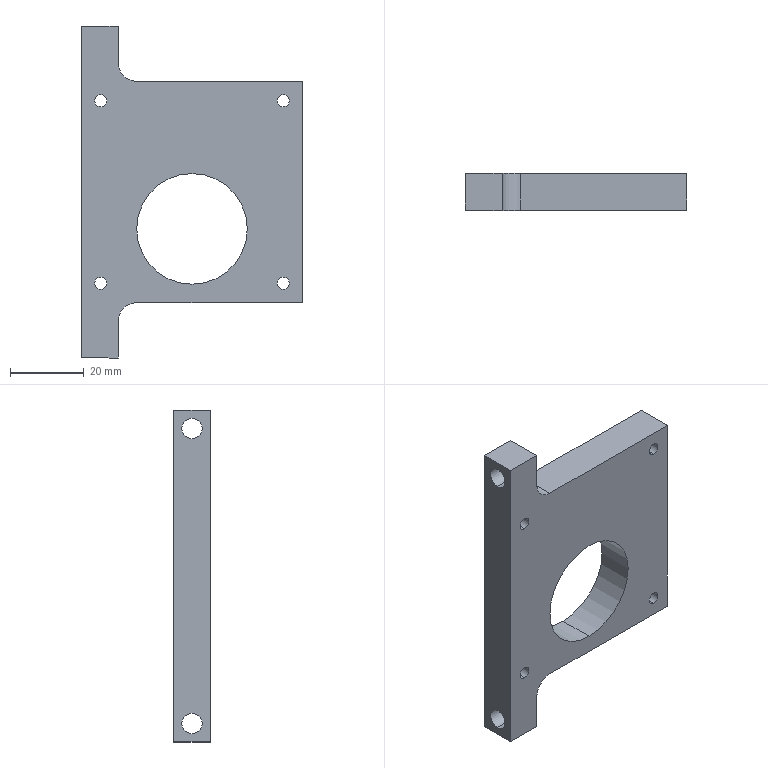Part | SolidWorks | features HoleWzd 3, Cut 1, Extrusion 1, Fillet 1, ICE 1, MoveFace 1 | 1 solid | 30 faces | box 60 x 10 x 90 mm | volume 31044 mm3 | cylinder 18 | plane 10 | cone 2 | commonest cylinder face diameters 3.3 x8 5.5 x4 4.2 x2 10 x2 30 x2
STEP:
#1=CARTESIAN_POINT('',(17.6,4.5,12.101));
#2=VERTEX_POINT('',#1);
#3=CARTESIAN_POINT('',(17.6,4.5,7.901));
#4=VERTEX_POINT('',#3);
#5=CARTESIAN_POINT('',(17.6,4.5,10.001));
#6=DIRECTION('',(1.,0.,0.));
#7=DIRECTION('',(0.,0.,-1.));
#8=AXIS2_PLACEMENT_3D('',#5,#6,#7);
#9=CIRCLE('',#8,2.1);
#10=EDGE_CURVE('',#2,#4,#9,.T.);
#11=ORIENTED_EDGE('',*,*,#10,.F.);
#12=CARTESIAN_POINT('',(30.,4.5,12.101));
#13=VERTEX_POINT('',#12);
#14=CARTESIAN_POINT('',(30.,4.5,12.101));
#15=DIRECTION('',(1.,0.,0.));
#16=VECTOR('',#15,1000.);
#17=LINE('',#14,#16);
#18=EDGE_CURVE('',#2,#13,#17,.T.);
#19=ORIENTED_EDGE('',*,*,#18,.T.);
#20=CARTESIAN_POINT('',(30.,4.5,7.901));
#21=VERTEX_POINT('',#20);
#22=CARTESIAN_POINT('',(30.,4.5,10.001));
#23=DIRECTION('',(1.,0.,0.));
#24=DIRECTION('',(0.,0.,-1.));
#25=AXIS2_PLACEMENT_3D('',#22,#23,#24);
#26=CIRCLE('',#25,2.1);
#27=EDGE_CURVE('',#13,#21,#26,.T.);
#28=ORIENTED_EDGE('',*,*,#27,.T.);
#29=CARTESIAN_POINT('',(30.,4.5,7.901));
#30=DIRECTION('',(1.,0.,0.));
#31=VECTOR('',#30,1000.);
#32=LINE('',#29,#31);
#33=EDGE_CURVE('',#4,#21,#32,.T.);
#34=ORIENTED_EDGE('',*,*,#33,.F.);
#35=EDGE_LOOP('',(#11,#19,#28,#34));
#36=FACE_OUTER_BOUND('',#35,.T.);
#37=CARTESIAN_POINT('',(30.,4.5,10.001));
#38=DIRECTION('',(1.,0.,0.));
#39=DIRECTION('',(0.,0.,-1.));
#40=AXIS2_PLACEMENT_3D('',#37,#38,#39);
#41=CYLINDRICAL_SURFACE('',#40,2.1);
#42=ADVANCED_FACE('',(#36),#41,.F.);
#43=CARTESIAN_POINT('',(16.338,4.5,10.001));
#44=VERTEX_POINT('',#43);
#45=CARTESIAN_POINT('',(17.6,4.5,7.901));
#46=DIRECTION('',(0.515,0.,-0.8572));
#47=VECTOR('',#46,1000.);
#48=LINE('',#45,#47);
#49=EDGE_CURVE('',#44,#4,#48,.T.);
#50=ORIENTED_EDGE('',*,*,#49,.F.);
#51=CARTESIAN_POINT('',(17.6,4.5,12.101));
#52=DIRECTION('',(0.515,0.,0.8572));
#53=VECTOR('',#52,1000.);
#54=LINE('',#51,#53);
#55=EDGE_CURVE('',#44,#2,#54,.T.);
#56=ORIENTED_EDGE('',*,*,#55,.T.);
#57=ORIENTED_EDGE('',*,*,#10,.T.);
#58=EDGE_LOOP('',(#50,#56,#57));
#59=FACE_OUTER_BOUND('',#58,.T.);
#60=CARTESIAN_POINT('',(17.6,4.5,10.001));
#61=DIRECTION('',(1.,0.,0.));
#62=DIRECTION('',(0.,0.,-1.));
#63=AXIS2_PLACEMENT_3D('',#60,#61,#62);
#64=CONICAL_SURFACE('',#63,2.1,1.03);
#65=ADVANCED_FACE('',(#59),#64,.F.);
#66=CARTESIAN_POINT('',(-20.,5.,-42.75));
#67=VERTEX_POINT('',#66);
#68=CARTESIAN_POINT('',(-20.,5.,-37.25));
#69=VERTEX_POINT('',#68);
#70=CARTESIAN_POINT('',(-20.,5.,-40.));
#71=DIRECTION('',(-1.,0.,0.));
#72=DIRECTION('',(0.,0.,1.));
#73=AXIS2_PLACEMENT_3D('',#70,#71,#72);
#74=CIRCLE('',#73,2.75);
#75=EDGE_CURVE('',#67,#69,#74,.T.);
#76=ORIENTED_EDGE('',*,*,#75,.F.);
#77=CARTESIAN_POINT('',(-30.,5.,-42.75));
#78=VERTEX_POINT('',#77);
#79=CARTESIAN_POINT('',(-30.,5.,-42.75));
#80=DIRECTION('',(-1.,0.,0.));
#81=VECTOR('',#80,1000.);
#82=LINE('',#79,#81);
#83=EDGE_CURVE('',#67,#78,#82,.T.);
#84=ORIENTED_EDGE('',*,*,#83,.T.);
#85=CARTESIAN_POINT('',(-30.,5.,-37.25));
#86=VERTEX_POINT('',#85);
#87=CARTESIAN_POINT('',(-30.,5.,-40.));
#88=DIRECTION('',(-1.,0.,0.));
#89=DIRECTION('',(0.,0.,1.));
#90=AXIS2_PLACEMENT_3D('',#87,#88,#89);
#91=CIRCLE('',#90,2.75);
#92=EDGE_CURVE('',#78,#86,#91,.T.);
#93=ORIENTED_EDGE('',*,*,#92,.T.);
#94=CARTESIAN_POINT('',(-30.,5.,-37.25));
#95=DIRECTION('',(-1.,0.,0.));
#96=VECTOR('',#95,1000.);
#97=LINE('',#94,#96);
#98=EDGE_CURVE('',#69,#86,#97,.T.);
#99=ORIENTED_EDGE('',*,*,#98,.F.);
#100=EDGE_LOOP('',(#76,#84,#93,#99));
#101=FACE_OUTER_BOUND('',#100,.T.);
#102=CARTESIAN_POINT('',(-30.,5.,-40.));
#103=DIRECTION('',(-1.,0.,0.));
#104=DIRECTION('',(0.,0.,1.));
#105=AXIS2_PLACEMENT_3D('',#102,#103,#104);
#106=CYLINDRICAL_SURFACE('',#105,2.75);
#107=ADVANCED_FACE('',(#101),#106,.F.);
#108=CARTESIAN_POINT('',(-20.,5.,37.25));
#109=VERTEX_POINT('',#108);
#110=CARTESIAN_POINT('',(-20.,5.,42.75));
#111=VERTEX_POINT('',#110);
#112=CARTESIAN_POINT('',(-20.,5.,40.));
#113=DIRECTION('',(-1.,0.,0.));
#114=DIRECTION('',(0.,0.,1.));
#115=AXIS2_PLACEMENT_3D('',#112,#113,#114);
#116=CIRCLE('',#115,2.75);
#117=EDGE_CURVE('',#109,#111,#116,.T.);
#118=ORIENTED_EDGE('',*,*,#117,.F.);
#119=CARTESIAN_POINT('',(-30.,5.,37.25));
#120=VERTEX_POINT('',#119);
#121=CARTESIAN_POINT('',(-30.,5.,37.25));
#122=DIRECTION('',(-1.,0.,0.));
#123=VECTOR('',#122,1000.);
#124=LINE('',#121,#123);
#125=EDGE_CURVE('',#109,#120,#124,.T.);
#126=ORIENTED_EDGE('',*,*,#125,.T.);
#127=CARTESIAN_POINT('',(-30.,5.,42.75));
#128=VERTEX_POINT('',#127);
#129=CARTESIAN_POINT('',(-30.,5.,40.));
#130=DIRECTION('',(-1.,0.,0.));
#131=DIRECTION('',(0.,0.,1.));
#132=AXIS2_PLACEMENT_3D('',#129,#130,#131);
#133=CIRCLE('',#132,2.75);
#134=EDGE_CURVE('',#120,#128,#133,.T.);
#135=ORIENTED_EDGE('',*,*,#134,.T.);
#136=CARTESIAN_POINT('',(-30.,5.,42.75));
#137=DIRECTION('',(-1.,0.,0.));
#138=VECTOR('',#137,1000.);
#139=LINE('',#136,#138);
#140=EDGE_CURVE('',#111,#128,#139,.T.);
#141=ORIENTED_EDGE('',*,*,#140,.F.);
#142=EDGE_LOOP('',(#118,#126,#135,#141));
#143=FACE_OUTER_BOUND('',#142,.T.);
#144=CARTESIAN_POINT('',(-30.,5.,40.));
#145=DIRECTION('',(-1.,0.,0.));
#146=DIRECTION('',(0.,0.,1.));
#147=AXIS2_PLACEMENT_3D('',#144,#145,#146);
#148=CYLINDRICAL_SURFACE('',#147,2.75);
#149=ADVANCED_FACE('',(#143),#148,.F.);
#150=CARTESIAN_POINT('',(-24.749,10.,26.397));
#151=VERTEX_POINT('',#150);
#152=CARTESIAN_POINT('',(-24.749,10.,23.097));
#153=VERTEX_POINT('',#152);
#154=CARTESIAN_POINT('',(-24.749,10.,24.747));
#155=DIRECTION('',(0.,-1.,0.));
#156=DIRECTION('',(0.,0.,-1.));
#157=AXIS2_PLACEMENT_3D('',#154,#155,#156);
#158=CIRCLE('',#157,1.65);
#159=EDGE_CURVE('',#151,#153,#158,.T.);
#160=ORIENTED_EDGE('',*,*,#159,.F.);
#161=CARTESIAN_POINT('',(-24.749,0.,26.397));
#162=VERTEX_POINT('',#161);
#163=CARTESIAN_POINT('',(-24.749,0.,26.397));
#164=DIRECTION('',(0.,-1.,0.));
#165=VECTOR('',#164,1000.);
#166=LINE('',#163,#165);
#167=EDGE_CURVE('',#151,#162,#166,.T.);
#168=ORIENTED_EDGE('',*,*,#167,.T.);
#169=CARTESIAN_POINT('',(-24.749,0.,23.097));
#170=VERTEX_POINT('',#169);
#171=CARTESIAN_POINT('',(-24.749,0.,24.747));
#172=DIRECTION('',(0.,-1.,0.));
#173=DIRECTION('',(0.,0.,-1.));
#174=AXIS2_PLACEMENT_3D('',#171,#172,#173);
#175=CIRCLE('',#174,1.65);
#176=EDGE_CURVE('',#162,#170,#175,.T.);
#177=ORIENTED_EDGE('',*,*,#176,.T.);
#178=CARTESIAN_POINT('',(-24.749,0.,23.097));
#179=DIRECTION('',(0.,-1.,0.));
#180=VECTOR('',#179,1000.);
#181=LINE('',#178,#180);
#182=EDGE_CURVE('',#153,#170,#181,.T.);
#183=ORIENTED_EDGE('',*,*,#182,.F.);
#184=EDGE_LOOP('',(#160,#168,#177,#183));
#185=FACE_OUTER_BOUND('',#184,.T.);
#186=CARTESIAN_POINT('',(-24.749,0.,24.747));
#187=DIRECTION('',(0.,-1.,0.));
#188=DIRECTION('',(0.,0.,-1.));
#189=AXIS2_PLACEMENT_3D('',#186,#187,#188);
#190=CYLINDRICAL_SURFACE('',#189,1.65);
#191=ADVANCED_FACE('',(#185),#190,.F.);
#192=CARTESIAN_POINT('',(-24.749,10.,-23.1));
#193=VERTEX_POINT('',#192);
#194=CARTESIAN_POINT('',(-24.749,10.,-26.4));
#195=VERTEX_POINT('',#194);
#196=CARTESIAN_POINT('',(-24.749,10.,-24.75));
#197=DIRECTION('',(0.,-1.,0.));
#198=DIRECTION('',(0.,0.,-1.));
#199=AXIS2_PLACEMENT_3D('',#196,#197,#198);
#200=CIRCLE('',#199,1.65);
#201=EDGE_CURVE('',#193,#195,#200,.T.);
#202=ORIENTED_EDGE('',*,*,#201,.F.);
#203=CARTESIAN_POINT('',(-24.749,0.,-23.1));
#204=VERTEX_POINT('',#203);
#205=CARTESIAN_POINT('',(-24.749,0.,-23.1));
#206=DIRECTION('',(0.,-1.,0.));
#207=VECTOR('',#206,1000.);
#208=LINE('',#205,#207);
#209=EDGE_CURVE('',#193,#204,#208,.T.);
#210=ORIENTED_EDGE('',*,*,#209,.T.);
#211=CARTESIAN_POINT('',(-24.749,0.,-26.4));
#212=VERTEX_POINT('',#211);
#213=CARTESIAN_POINT('',(-24.749,0.,-24.75));
#214=DIRECTION('',(0.,-1.,0.));
#215=DIRECTION('',(0.,0.,-1.));
#216=AXIS2_PLACEMENT_3D('',#213,#214,#215);
#217=CIRCLE('',#216,1.65);
#218=EDGE_CURVE('',#204,#212,#217,.T.);
#219=ORIENTED_EDGE('',*,*,#218,.T.);
#220=CARTESIAN_POINT('',(-24.749,0.,-26.4));
#221=DIRECTION('',(0.,-1.,0.));
#222=VECTOR('',#221,1000.);
#223=LINE('',#220,#222);
#224=EDGE_CURVE('',#195,#212,#223,.T.);
#225=ORIENTED_EDGE('',*,*,#224,.F.);
#226=EDGE_LOOP('',(#202,#210,#219,#225));
#227=FACE_OUTER_BOUND('',#226,.T.);
#228=CARTESIAN_POINT('',(-24.749,0.,-24.75));
#229=DIRECTION('',(0.,-1.,0.));
#230=DIRECTION('',(0.,0.,-1.));
#231=AXIS2_PLACEMENT_3D('',#228,#229,#230);
#232=CYLINDRICAL_SURFACE('',#231,1.65);
#233=ADVANCED_FACE('',(#227),#232,.F.);
#234=CARTESIAN_POINT('',(24.749,10.,-23.1));
#235=VERTEX_POINT('',#234);
#236=CARTESIAN_POINT('',(24.749,10.,-26.4));
#237=VERTEX_POINT('',#236);
#238=CARTESIAN_POINT('',(24.749,10.,-24.75));
#239=DIRECTION('',(0.,-1.,0.));
#240=DIRECTION('',(0.,0.,-1.));
#241=AXIS2_PLACEMENT_3D('',#238,#239,#240);
#242=CIRCLE('',#241,1.65);
#243=EDGE_CURVE('',#235,#237,#242,.T.);
#244=ORIENTED_EDGE('',*,*,#243,.F.);
#245=CARTESIAN_POINT('',(24.749,0.,-23.1));
#246=VERTEX_POINT('',#245);
#247=CARTESIAN_POINT('',(24.749,0.,-23.1));
#248=DIRECTION('',(0.,-1.,0.));
#249=VECTOR('',#248,1000.);
#250=LINE('',#247,#249);
#251=EDGE_CURVE('',#235,#246,#250,.T.);
#252=ORIENTED_EDGE('',*,*,#251,.T.);
#253=CARTESIAN_POINT('',(24.749,0.,-26.4));
#254=VERTEX_POINT('',#253);
#255=CARTESIAN_POINT('',(24.749,0.,-24.75));
#256=DIRECTION('',(0.,-1.,0.));
#257=DIRECTION('',(0.,0.,-1.));
#258=AXIS2_PLACEMENT_3D('',#255,#256,#257);
#259=CIRCLE('',#258,1.65);
#260=EDGE_CURVE('',#246,#254,#259,.T.);
#261=ORIENTED_EDGE('',*,*,#260,.T.);
#262=CARTESIAN_POINT('',(24.749,0.,-26.4));
#263=DIRECTION('',(0.,-1.,0.));
#264=VECTOR('',#263,1000.);
#265=LINE('',#262,#264);
#266=EDGE_CURVE('',#237,#254,#265,.T.);
#267=ORIENTED_EDGE('',*,*,#266,.F.);
#268=EDGE_LOOP('',(#244,#252,#261,#267));
#269=FACE_OUTER_BOUND('',#268,.T.);
#270=CARTESIAN_POINT('',(24.749,0.,-24.75));
#271=DIRECTION('',(0.,-1.,0.));
#272=DIRECTION('',(0.,0.,-1.));
#273=AXIS2_PLACEMENT_3D('',#270,#271,#272);
#274=CYLINDRICAL_SURFACE('',#273,1.65);
#275=ADVANCED_FACE('',(#269),#274,.F.);
#276=CARTESIAN_POINT('',(24.749,10.,26.397));
#277=VERTEX_POINT('',#276);
#278=CARTESIAN_POINT('',(24.749,10.,23.097));
#279=VERTEX_POINT('',#278);
#280=CARTESIAN_POINT('',(24.749,10.,24.747));
#281=DIRECTION('',(0.,-1.,0.));
#282=DIRECTION('',(0.,0.,-1.));
#283=AXIS2_PLACEMENT_3D('',#280,#281,#282);
#284=CIRCLE('',#283,1.65);
#285=EDGE_CURVE('',#277,#279,#284,.T.);
#286=ORIENTED_EDGE('',*,*,#285,.F.);
#287=CARTESIAN_POINT('',(24.749,0.,26.397));
#288=VERTEX_POINT('',#287);
#289=CARTESIAN_POINT('',(24.749,0.,26.397));
#290=DIRECTION('',(0.,-1.,0.));
#291=VECTOR('',#290,1000.);
#292=LINE('',#289,#291);
#293=EDGE_CURVE('',#277,#288,#292,.T.);
#294=ORIENTED_EDGE('',*,*,#293,.T.);
#295=CARTESIAN_POINT('',(24.749,0.,23.097));
#296=VERTEX_POINT('',#295);
#297=CARTESIAN_POINT('',(24.749,0.,24.747));
#298=DIRECTION('',(0.,-1.,0.));
#299=DIRECTION('',(0.,0.,-1.));
#300=AXIS2_PLACEMENT_3D('',#297,#298,#299);
#301=CIRCLE('',#300,1.65);
#302=EDGE_CURVE('',#288,#296,#301,.T.);
#303=ORIENTED_EDGE('',*,*,#302,.T.);
#304=CARTESIAN_POINT('',(24.749,0.,23.097));
#305=DIRECTION('',(0.,-1.,0.));
#306=VECTOR('',#305,1000.);
#307=LINE('',#304,#306);
#308=EDGE_CURVE('',#279,#296,#307,.T.);
#309=ORIENTED_EDGE('',*,*,#308,.F.);
#310=EDGE_LOOP('',(#286,#294,#303,#309));
#311=FACE_OUTER_BOUND('',#310,.T.);
#312=CARTESIAN_POINT('',(24.749,0.,24.747));
#313=DIRECTION('',(0.,-1.,0.));
#314=DIRECTION('',(0.,0.,-1.));
#315=AXIS2_PLACEMENT_3D('',#312,#313,#314);
#316=CYLINDRICAL_SURFACE('',#315,1.65);
#317=ADVANCED_FACE('',(#311),#316,.F.);
#318=CARTESIAN_POINT('',(0.,10.,5.));
#319=VERTEX_POINT('',#318);
#320=CARTESIAN_POINT('',(0.,10.,-25.));
#321=VERTEX_POINT('',#320);
#322=CARTESIAN_POINT('',(0.,10.,-10.));
#323=DIRECTION('',(0.,-1.,0.));
#324=DIRECTION('',(0.,0.,-1.));
#325=AXIS2_PLACEMENT_3D('',#322,#323,#324);
#326=CIRCLE('',#325,15.);
#327=EDGE_CURVE('',#319,#321,#326,.T.);
#328=ORIENTED_EDGE('',*,*,#327,.F.);
#329=CARTESIAN_POINT('',(0.,0.,5.));
#330=VERTEX_POINT('',#329);
#331=CARTESIAN_POINT('',(0.,10.,5.));
#332=DIRECTION('',(0.,-1.,0.));
#333=VECTOR('',#332,1000.);
#334=LINE('',#331,#333);
#335=EDGE_CURVE('',#319,#330,#334,.T.);
#336=ORIENTED_EDGE('',*,*,#335,.T.);
#337=CARTESIAN_POINT('',(0.,0.,-25.));
#338=VERTEX_POINT('',#337);
#339=CARTESIAN_POINT('',(0.,0.,-10.));
#340=DIRECTION('',(0.,-1.,0.));
#341=DIRECTION('',(0.,0.,-1.));
#342=AXIS2_PLACEMENT_3D('',#339,#340,#341);
#343=CIRCLE('',#342,15.);
#344=EDGE_CURVE('',#330,#338,#343,.T.);
#345=ORIENTED_EDGE('',*,*,#344,.T.);
#346=CARTESIAN_POINT('',(0.,10.,-25.));
#347=DIRECTION('',(0.,-1.,0.));
#348=VECTOR('',#347,1000.);
#349=LINE('',#346,#348);
#350=EDGE_CURVE('',#321,#338,#349,.T.);
#351=ORIENTED_EDGE('',*,*,#350,.F.);
#352=EDGE_LOOP('',(#328,#336,#345,#351));
#353=FACE_OUTER_BOUND('',#352,.T.);
#354=CARTESIAN_POINT('',(0.,10.,-10.));
#355=DIRECTION('',(0.,-1.,0.));
#356=DIRECTION('',(0.,0.,-1.));
#357=AXIS2_PLACEMENT_3D('',#354,#355,#356);
#358=CYLINDRICAL_SURFACE('',#357,15.);
#359=ADVANCED_FACE('',(#353),#358,.F.);
#360=CARTESIAN_POINT('',(-30.,5.,-40.));
#361=DIRECTION('',(-1.,0.,0.));
#362=DIRECTION('',(0.,0.,1.));
#363=AXIS2_PLACEMENT_3D('',#360,#361,#362);
#364=CIRCLE('',#363,2.75);
#365=EDGE_CURVE('',#86,#78,#364,.T.);
#366=ORIENTED_EDGE('',*,*,#365,.F.);
#367=ORIENTED_EDGE('',*,*,#92,.F.);
#368=EDGE_LOOP('',(#366,#367));
#369=FACE_BOUND('',#368,.T.);
#370=CARTESIAN_POINT('',(-30.,5.,40.));
#371=DIRECTION('',(-1.,0.,0.));
#372=DIRECTION('',(0.,0.,1.));
#373=AXIS2_PLACEMENT_3D('',#370,#371,#372);
#374=CIRCLE('',#373,2.75);
#375=EDGE_CURVE('',#128,#120,#374,.T.);
#376=ORIENTED_EDGE('',*,*,#375,.F.);
#377=ORIENTED_EDGE('',*,*,#134,.F.);
#378=EDGE_LOOP('',(#376,#377));
#379=FACE_BOUND('',#378,.T.);
#380=CARTESIAN_POINT('',(-30.,0.,-45.));
#381=VERTEX_POINT('',#380);
#382=CARTESIAN_POINT('',(-30.,0.,45.));
#383=VERTEX_POINT('',#382);
#384=CARTESIAN_POINT('',(-30.,0.,45.));
#385=DIRECTION('',(0.,0.,1.));
#386=VECTOR('',#385,1000.);
#387=LINE('',#384,#386);
#388=EDGE_CURVE('',#381,#383,#387,.T.);
#389=ORIENTED_EDGE('',*,*,#388,.T.);
#390=CARTESIAN_POINT('',(-30.,10.,45.));
#391=VERTEX_POINT('',#390);
#392=CARTESIAN_POINT('',(-30.,10.,45.));
#393=DIRECTION('',(0.,-1.,0.));
#394=VECTOR('',#393,1000.);
#395=LINE('',#392,#394);
#396=EDGE_CURVE('',#391,#383,#395,.T.);
#397=ORIENTED_EDGE('',*,*,#396,.F.);
#398=CARTESIAN_POINT('',(-30.,10.,-45.));
#399=VERTEX_POINT('',#398);
#400=CARTESIAN_POINT('',(-30.,10.,45.));
#401=DIRECTION('',(0.,0.,1.));
#402=VECTOR('',#401,1000.);
#403=LINE('',#400,#402);
#404=EDGE_CURVE('',#399,#391,#403,.T.);
#405=ORIENTED_EDGE('',*,*,#404,.F.);
#406=CARTESIAN_POINT('',(-30.,10.,-45.));
#407=DIRECTION('',(0.,-1.,0.));
#408=VECTOR('',#407,1000.);
#409=LINE('',#406,#408);
#410=EDGE_CURVE('',#399,#381,#409,.T.);
#411=ORIENTED_EDGE('',*,*,#410,.T.);
#412=EDGE_LOOP('',(#389,#397,#405,#411));
#413=FACE_OUTER_BOUND('',#412,.T.);
#414=CARTESIAN_POINT('',(-30.,10.,45.));
#415=DIRECTION('',(1.,0.,0.));
#416=DIRECTION('',(0.,0.,-1.));
#417=AXIS2_PLACEMENT_3D('',#414,#415,#416);
#418=PLANE('',#417);
#419=ADVANCED_FACE('',(#369,#379,#413),#418,.F.);
#420=CARTESIAN_POINT('',(-20.,0.,45.));
#421=VERTEX_POINT('',#420);
#422=CARTESIAN_POINT('',(30.,0.,45.));
#423=DIRECTION('',(1.,0.,0.));
#424=VECTOR('',#423,1000.);
#425=LINE('',#422,#424);
#426=EDGE_CURVE('',#383,#421,#425,.T.);
#427=ORIENTED_EDGE('',*,*,#426,.T.);
#428=CARTESIAN_POINT('',(-20.,10.,45.));
#429=VERTEX_POINT('',#428);
#430=CARTESIAN_POINT('',(-20.,10.,45.));
#431=DIRECTION('',(0.,-1.,0.));
#432=VECTOR('',#431,1000.);
#433=LINE('',#430,#432);
#434=EDGE_CURVE('',#429,#421,#433,.T.);
#435=ORIENTED_EDGE('',*,*,#434,.F.);
#436=CARTESIAN_POINT('',(30.,10.,45.));
#437=DIRECTION('',(1.,0.,0.));
#438=VECTOR('',#437,1000.);
#439=LINE('',#436,#438);
#440=EDGE_CURVE('',#391,#429,#439,.T.);
#441=ORIENTED_EDGE('',*,*,#440,.F.);
#442=ORIENTED_EDGE('',*,*,#396,.T.);
#443=EDGE_LOOP('',(#427,#435,#441,#442));
#444=FACE_OUTER_BOUND('',#443,.T.);
#445=CARTESIAN_POINT('',(30.,10.,45.));
#446=DIRECTION('',(0.,0.,-1.));
#447=DIRECTION('',(-1.,0.,0.));
#448=AXIS2_PLACEMENT_3D('',#445,#446,#447);
#449=PLANE('',#448);
#450=ADVANCED_FACE('',(#444),#449,.F.);
#451=CARTESIAN_POINT('',(30.,4.5,10.001));
#452=DIRECTION('',(1.,0.,0.));
#453=DIRECTION('',(0.,0.,-1.));
#454=AXIS2_PLACEMENT_3D('',#451,#452,#453);
#455=CIRCLE('',#454,2.1);
#456=EDGE_CURVE('',#21,#13,#455,.T.);
#457=ORIENTED_EDGE('',*,*,#456,.F.);
#458=ORIENTED_EDGE('',*,*,#27,.F.);
#459=EDGE_LOOP('',(#457,#458));
#460=FACE_BOUND('',#459,.T.);
#461=CARTESIAN_POINT('',(30.,10.,30.));
#462=VERTEX_POINT('',#461);
#463=CARTESIAN_POINT('',(30.,10.,-30.));
#464=VERTEX_POINT('',#463);
#465=CARTESIAN_POINT('',(30.,10.,45.));
#466=DIRECTION('',(0.,0.,-1.));
#467=VECTOR('',#466,1000.);
#468=LINE('',#465,#467);
#469=EDGE_CURVE('',#462,#464,#468,.T.);
#470=ORIENTED_EDGE('',*,*,#469,.F.);
#471=CARTESIAN_POINT('',(30.,0.,30.));
#472=VERTEX_POINT('',#471);
#473=CARTESIAN_POINT('',(30.,10.,30.));
#474=DIRECTION('',(0.,-1.,0.));
#475=VECTOR('',#474,1000.);
#476=LINE('',#473,#475);
#477=EDGE_CURVE('',#462,#472,#476,.T.);
#478=ORIENTED_EDGE('',*,*,#477,.T.);
#479=CARTESIAN_POINT('',(30.,0.,-30.));
#480=VERTEX_POINT('',#479);
#481=CARTESIAN_POINT('',(30.,0.,45.));
#482=DIRECTION('',(0.,0.,-1.));
#483=VECTOR('',#482,1000.);
#484=LINE('',#481,#483);
#485=EDGE_CURVE('',#472,#480,#484,.T.);
#486=ORIENTED_EDGE('',*,*,#485,.T.);
#487=CARTESIAN_POINT('',(30.,10.,-30.));
#488=DIRECTION('',(0.,-1.,0.));
#489=VECTOR('',#488,1000.);
#490=LINE('',#487,#489);
#491=EDGE_CURVE('',#464,#480,#490,.T.);
#492=ORIENTED_EDGE('',*,*,#491,.F.);
#493=EDGE_LOOP('',(#470,#478,#486,#492));
#494=FACE_OUTER_BOUND('',#493,.T.);
#495=CARTESIAN_POINT('',(30.,10.,45.));
#496=DIRECTION('',(-1.,0.,0.));
#497=DIRECTION('',(0.,0.,1.));
#498=AXIS2_PLACEMENT_3D('',#495,#496,#497);
#499=PLANE('',#498);
#500=ADVANCED_FACE('',(#460,#494),#499,.F.);
#501=CARTESIAN_POINT('',(-20.,10.,-45.));
#502=VERTEX_POINT('',#501);
#503=CARTESIAN_POINT('',(30.,10.,-45.));
#504=DIRECTION('',(-1.,0.,0.));
#505=VECTOR('',#504,1000.);
#506=LINE('',#503,#505);
#507=EDGE_CURVE('',#502,#399,#506,.T.);
#508=ORIENTED_EDGE('',*,*,#507,.F.);
#509=CARTESIAN_POINT('',(-20.,0.,-45.));
#510=VERTEX_POINT('',#509);
#511=CARTESIAN_POINT('',(-20.,10.,-45.));
#512=DIRECTION('',(0.,-1.,0.));
#513=VECTOR('',#512,1000.);
#514=LINE('',#511,#513);
#515=EDGE_CURVE('',#502,#510,#514,.T.);
#516=ORIENTED_EDGE('',*,*,#515,.T.);
#517=CARTESIAN_POINT('',(30.,0.,-45.));
#518=DIRECTION('',(-1.,0.,0.));
#519=VECTOR('',#518,1000.);
#520=LINE('',#517,#519);
#521=EDGE_CURVE('',#510,#381,#520,.T.);
#522=ORIENTED_EDGE('',*,*,#521,.T.);
#523=ORIENTED_EDGE('',*,*,#410,.F.);
#524=EDGE_LOOP('',(#508,#516,#522,#523));
#525=FACE_OUTER_BOUND('',#524,.T.);
#526=CARTESIAN_POINT('',(30.,10.,-45.));
#527=DIRECTION('',(0.,0.,1.));
#528=DIRECTION('',(1.,0.,0.));
#529=AXIS2_PLACEMENT_3D('',#526,#527,#528);
#530=PLANE('',#529);
#531=ADVANCED_FACE('',(#525),#530,.F.);
#532=CARTESIAN_POINT('',(-20.,10.,35.));
#533=VERTEX_POINT('',#532);
#534=CARTESIAN_POINT('',(-20.,10.,45.));
#535=DIRECTION('',(0.,0.,-1.));
#536=VECTOR('',#535,1000.);
#537=LINE('',#534,#536);
#538=EDGE_CURVE('',#429,#533,#537,.T.);
#539=ORIENTED_EDGE('',*,*,#538,.T.);
#540=CARTESIAN_POINT('',(-15.,10.,30.));
#541=VERTEX_POINT('',#540);
#542=CARTESIAN_POINT('',(-15.,10.,35.));
#543=DIRECTION('',(0.,-1.,0.));
#544=DIRECTION('',(0.,0.,1.));
#545=AXIS2_PLACEMENT_3D('',#542,#543,#544);
#546=CIRCLE('',#545,5.);
#547=EDGE_CURVE('',#533,#541,#546,.T.);
#548=ORIENTED_EDGE('',*,*,#547,.T.);
#549=CARTESIAN_POINT('',(30.,10.,30.));
#550=DIRECTION('',(1.,0.,0.));
#551=VECTOR('',#550,1000.);
#552=LINE('',#549,#551);
#553=EDGE_CURVE('',#541,#462,#552,.T.);
#554=ORIENTED_EDGE('',*,*,#553,.T.);
#555=ORIENTED_EDGE('',*,*,#469,.T.);
#556=CARTESIAN_POINT('',(-15.,10.,-30.));
#557=VERTEX_POINT('',#556);
#558=CARTESIAN_POINT('',(30.,10.,-30.));
#559=DIRECTION('',(-1.,0.,0.));
#560=VECTOR('',#559,1000.);
#561=LINE('',#558,#560);
#562=EDGE_CURVE('',#464,#557,#561,.T.);
#563=ORIENTED_EDGE('',*,*,#562,.T.);
#564=CARTESIAN_POINT('',(-20.,10.,-35.));
#565=VERTEX_POINT('',#564);
#566=CARTESIAN_POINT('',(-15.,10.,-35.));
#567=DIRECTION('',(0.,-1.,0.));
#568=DIRECTION('',(0.,0.,1.));
#569=AXIS2_PLACEMENT_3D('',#566,#567,#568);
#570=CIRCLE('',#569,5.);
#571=EDGE_CURVE('',#557,#565,#570,.T.);
#572=ORIENTED_EDGE('',*,*,#571,.T.);
#573=CARTESIAN_POINT('',(-20.,10.,-45.));
#574=DIRECTION('',(0.,0.,-1.));
#575=VECTOR('',#574,1000.);
#576=LINE('',#573,#575);
#577=EDGE_CURVE('',#565,#502,#576,.T.);
#578=ORIENTED_EDGE('',*,*,#577,.T.);
#579=ORIENTED_EDGE('',*,*,#507,.T.);
#580=ORIENTED_EDGE('',*,*,#404,.T.);
#581=ORIENTED_EDGE('',*,*,#440,.T.);
#582=EDGE_LOOP('',(#539,#548,#554,#555,#563,#572,#578,#579,#580,#581));
#583=FACE_OUTER_BOUND('',#582,.T.);
#584=CARTESIAN_POINT('',(-24.749,10.,24.747));
#585=DIRECTION('',(0.,-1.,0.));
#586=DIRECTION('',(0.,0.,-1.));
#587=AXIS2_PLACEMENT_3D('',#584,#585,#586);
#588=CIRCLE('',#587,1.65);
#589=EDGE_CURVE('',#153,#151,#588,.T.);
#590=ORIENTED_EDGE('',*,*,#589,.T.);
#591=ORIENTED_EDGE('',*,*,#159,.T.);
#592=EDGE_LOOP('',(#590,#591));
#593=FACE_BOUND('',#592,.T.);
#594=CARTESIAN_POINT('',(-24.749,10.,-24.75));
#595=DIRECTION('',(0.,-1.,0.));
#596=DIRECTION('',(0.,0.,-1.));
#597=AXIS2_PLACEMENT_3D('',#594,#595,#596);
#598=CIRCLE('',#597,1.65);
#599=EDGE_CURVE('',#195,#193,#598,.T.);
#600=ORIENTED_EDGE('',*,*,#599,.T.);
#601=ORIENTED_EDGE('',*,*,#201,.T.);
#602=EDGE_LOOP('',(#600,#601));
#603=FACE_BOUND('',#602,.T.);
#604=CARTESIAN_POINT('',(24.749,10.,-24.75));
#605=DIRECTION('',(0.,-1.,0.));
#606=DIRECTION('',(0.,0.,-1.));
#607=AXIS2_PLACEMENT_3D('',#604,#605,#606);
#608=CIRCLE('',#607,1.65);
#609=EDGE_CURVE('',#237,#235,#608,.T.);
#610=ORIENTED_EDGE('',*,*,#609,.T.);
#611=ORIENTED_EDGE('',*,*,#243,.T.);
#612=EDGE_LOOP('',(#610,#611));
#613=FACE_BOUND('',#612,.T.);
#614=CARTESIAN_POINT('',(24.749,10.,24.747));
#615=DIRECTION('',(0.,-1.,0.));
#616=DIRECTION('',(0.,0.,-1.));
#617=AXIS2_PLACEMENT_3D('',#614,#615,#616);
#618=CIRCLE('',#617,1.65);
#619=EDGE_CURVE('',#279,#277,#618,.T.);
#620=ORIENTED_EDGE('',*,*,#619,.T.);
#621=ORIENTED_EDGE('',*,*,#285,.T.);
#622=EDGE_LOOP('',(#620,#621));
#623=FACE_BOUND('',#622,.T.);
#624=CARTESIAN_POINT('',(0.,10.,-10.));
#625=DIRECTION('',(0.,-1.,0.));
#626=DIRECTION('',(0.,0.,-1.));
#627=AXIS2_PLACEMENT_3D('',#624,#625,#626);
#628=CIRCLE('',#627,15.);
#629=EDGE_CURVE('',#321,#319,#628,.T.);
#630=ORIENTED_EDGE('',*,*,#629,.T.);
#631=ORIENTED_EDGE('',*,*,#327,.T.);
#632=EDGE_LOOP('',(#630,#631));
#633=FACE_BOUND('',#632,.T.);
#634=CARTESIAN_POINT('',(0.,10.,0.));
#635=DIRECTION('',(0.,1.,0.));
#636=DIRECTION('',(0.,0.,1.));
#637=AXIS2_PLACEMENT_3D('',#634,#635,#636);
#638=PLANE('',#637);
#639=ADVANCED_FACE('',(#583,#593,#603,#613,#623,#633),#638,.T.);
#640=CARTESIAN_POINT('',(-24.749,0.,24.747));
#641=DIRECTION('',(0.,-1.,0.));
#642=DIRECTION('',(0.,0.,-1.));
#643=AXIS2_PLACEMENT_3D('',#640,#641,#642);
#644=CIRCLE('',#643,1.65);
#645=EDGE_CURVE('',#170,#162,#644,.T.);
#646=ORIENTED_EDGE('',*,*,#645,.F.);
#647=ORIENTED_EDGE('',*,*,#176,.F.);
#648=EDGE_LOOP('',(#646,#647));
#649=FACE_BOUND('',#648,.T.);
#650=CARTESIAN_POINT('',(-24.749,0.,-24.75));
#651=DIRECTION('',(0.,-1.,0.));
#652=DIRECTION('',(0.,0.,-1.));
#653=AXIS2_PLACEMENT_3D('',#650,#651,#652);
#654=CIRCLE('',#653,1.65);
#655=EDGE_CURVE('',#212,#204,#654,.T.);
#656=ORIENTED_EDGE('',*,*,#655,.F.);
#657=ORIENTED_EDGE('',*,*,#218,.F.);
#658=EDGE_LOOP('',(#656,#657));
#659=FACE_BOUND('',#658,.T.);
#660=CARTESIAN_POINT('',(24.749,0.,-24.75));
#661=DIRECTION('',(0.,-1.,0.));
#662=DIRECTION('',(0.,0.,-1.));
#663=AXIS2_PLACEMENT_3D('',#660,#661,#662);
#664=CIRCLE('',#663,1.65);
#665=EDGE_CURVE('',#254,#246,#664,.T.);
#666=ORIENTED_EDGE('',*,*,#665,.F.);
#667=ORIENTED_EDGE('',*,*,#260,.F.);
#668=EDGE_LOOP('',(#666,#667));
#669=FACE_BOUND('',#668,.T.);
#670=CARTESIAN_POINT('',(24.749,0.,24.747));
#671=DIRECTION('',(0.,-1.,0.));
#672=DIRECTION('',(0.,0.,-1.));
#673=AXIS2_PLACEMENT_3D('',#670,#671,#672);
#674=CIRCLE('',#673,1.65);
#675=EDGE_CURVE('',#296,#288,#674,.T.);
#676=ORIENTED_EDGE('',*,*,#675,.F.);
#677=ORIENTED_EDGE('',*,*,#302,.F.);
#678=EDGE_LOOP('',(#676,#677));
#679=FACE_BOUND('',#678,.T.);
#680=CARTESIAN_POINT('',(0.,0.,-10.));
#681=DIRECTION('',(0.,-1.,0.));
#682=DIRECTION('',(0.,0.,-1.));
#683=AXIS2_PLACEMENT_3D('',#680,#681,#682);
#684=CIRCLE('',#683,15.);
#685=EDGE_CURVE('',#338,#330,#684,.T.);
#686=ORIENTED_EDGE('',*,*,#685,.F.);
#687=ORIENTED_EDGE('',*,*,#344,.F.);
#688=EDGE_LOOP('',(#686,#687));
#689=FACE_BOUND('',#688,.T.);
#690=ORIENTED_EDGE('',*,*,#485,.F.);
#691=CARTESIAN_POINT('',(-15.,0.,30.));
#692=VERTEX_POINT('',#691);
#693=CARTESIAN_POINT('',(30.,0.,30.));
#694=DIRECTION('',(1.,0.,0.));
#695=VECTOR('',#694,1000.);
#696=LINE('',#693,#695);
#697=EDGE_CURVE('',#692,#472,#696,.T.);
#698=ORIENTED_EDGE('',*,*,#697,.F.);
#699=CARTESIAN_POINT('',(-20.,0.,35.));
#700=VERTEX_POINT('',#699);
#701=CARTESIAN_POINT('',(-15.,0.,35.));
#702=DIRECTION('',(0.,1.,0.));
#703=DIRECTION('',(0.,0.,1.));
#704=AXIS2_PLACEMENT_3D('',#701,#702,#703);
#705=CIRCLE('',#704,5.);
#706=EDGE_CURVE('',#692,#700,#705,.T.);
#707=ORIENTED_EDGE('',*,*,#706,.T.);
#708=CARTESIAN_POINT('',(-20.,0.,45.));
#709=DIRECTION('',(0.,0.,-1.));
#710=VECTOR('',#709,1000.);
#711=LINE('',#708,#710);
#712=EDGE_CURVE('',#421,#700,#711,.T.);
#713=ORIENTED_EDGE('',*,*,#712,.F.);
#714=ORIENTED_EDGE('',*,*,#426,.F.);
#715=ORIENTED_EDGE('',*,*,#388,.F.);
#716=ORIENTED_EDGE('',*,*,#521,.F.);
#717=CARTESIAN_POINT('',(-20.,0.,-35.));
#718=VERTEX_POINT('',#717);
#719=CARTESIAN_POINT('',(-20.,0.,-45.));
#720=DIRECTION('',(0.,0.,-1.));
#721=VECTOR('',#720,1000.);
#722=LINE('',#719,#721);
#723=EDGE_CURVE('',#718,#510,#722,.T.);
#724=ORIENTED_EDGE('',*,*,#723,.F.);
#725=CARTESIAN_POINT('',(-15.,0.,-30.));
#726=VERTEX_POINT('',#725);
#727=CARTESIAN_POINT('',(-15.,0.,-35.));
#728=DIRECTION('',(0.,1.,0.));
#729=DIRECTION('',(0.,0.,1.));
#730=AXIS2_PLACEMENT_3D('',#727,#728,#729);
#731=CIRCLE('',#730,5.);
#732=EDGE_CURVE('',#718,#726,#731,.T.);
#733=ORIENTED_EDGE('',*,*,#732,.T.);
#734=CARTESIAN_POINT('',(30.,0.,-30.));
#735=DIRECTION('',(-1.,0.,0.));
#736=VECTOR('',#735,1000.);
#737=LINE('',#734,#736);
#738=EDGE_CURVE('',#480,#726,#737,.T.);
#739=ORIENTED_EDGE('',*,*,#738,.F.);
#740=EDGE_LOOP('',(#690,#698,#707,#713,#714,#715,#716,#724,#733,#739));
#741=FACE_OUTER_BOUND('',#740,.T.);
#742=CARTESIAN_POINT('',(0.,0.,0.));
#743=DIRECTION('',(0.,1.,0.));
#744=DIRECTION('',(0.,0.,1.));
#745=AXIS2_PLACEMENT_3D('',#742,#743,#744);
#746=PLANE('',#745);
#747=ADVANCED_FACE('',(#649,#659,#669,#679,#689,#741),#746,.F.);
#748=ORIENTED_EDGE('',*,*,#335,.F.);
#749=ORIENTED_EDGE('',*,*,#629,.F.);
#750=ORIENTED_EDGE('',*,*,#350,.T.);
#751=ORIENTED_EDGE('',*,*,#685,.T.);
#752=EDGE_LOOP('',(#748,#749,#750,#751));
#753=FACE_OUTER_BOUND('',#752,.T.);
#754=CARTESIAN_POINT('',(0.,10.,-10.));
#755=DIRECTION('',(0.,-1.,0.));
#756=DIRECTION('',(0.,0.,-1.));
#757=AXIS2_PLACEMENT_3D('',#754,#755,#756);
#758=CYLINDRICAL_SURFACE('',#757,15.);
#759=ADVANCED_FACE('',(#753),#758,.F.);
#760=ORIENTED_EDGE('',*,*,#293,.F.);
#761=ORIENTED_EDGE('',*,*,#619,.F.);
#762=ORIENTED_EDGE('',*,*,#308,.T.);
#763=ORIENTED_EDGE('',*,*,#675,.T.);
#764=EDGE_LOOP('',(#760,#761,#762,#763));
#765=FACE_OUTER_BOUND('',#764,.T.);
#766=CARTESIAN_POINT('',(24.749,0.,24.747));
#767=DIRECTION('',(0.,-1.,0.));
#768=DIRECTION('',(0.,0.,-1.));
#769=AXIS2_PLACEMENT_3D('',#766,#767,#768);
#770=CYLINDRICAL_SURFACE('',#769,1.65);
#771=ADVANCED_FACE('',(#765),#770,.F.);
#772=ORIENTED_EDGE('',*,*,#251,.F.);
#773=ORIENTED_EDGE('',*,*,#609,.F.);
#774=ORIENTED_EDGE('',*,*,#266,.T.);
#775=ORIENTED_EDGE('',*,*,#665,.T.);
#776=EDGE_LOOP('',(#772,#773,#774,#775));
#777=FACE_OUTER_BOUND('',#776,.T.);
#778=CARTESIAN_POINT('',(24.749,0.,-24.75));
#779=DIRECTION('',(0.,-1.,0.));
#780=DIRECTION('',(0.,0.,-1.));
#781=AXIS2_PLACEMENT_3D('',#778,#779,#780);
#782=CYLINDRICAL_SURFACE('',#781,1.65);
#783=ADVANCED_FACE('',(#777),#782,.F.);
#784=ORIENTED_EDGE('',*,*,#209,.F.);
#785=ORIENTED_EDGE('',*,*,#599,.F.);
#786=ORIENTED_EDGE('',*,*,#224,.T.);
#787=ORIENTED_EDGE('',*,*,#655,.T.);
#788=EDGE_LOOP('',(#784,#785,#786,#787));
#789=FACE_OUTER_BOUND('',#788,.T.);
#790=CARTESIAN_POINT('',(-24.749,0.,-24.75));
#791=DIRECTION('',(0.,-1.,0.));
#792=DIRECTION('',(0.,0.,-1.));
#793=AXIS2_PLACEMENT_3D('',#790,#791,#792);
#794=CYLINDRICAL_SURFACE('',#793,1.65);
#795=ADVANCED_FACE('',(#789),#794,.F.);
#796=ORIENTED_EDGE('',*,*,#167,.F.);
#797=ORIENTED_EDGE('',*,*,#589,.F.);
#798=ORIENTED_EDGE('',*,*,#182,.T.);
#799=ORIENTED_EDGE('',*,*,#645,.T.);
#800=EDGE_LOOP('',(#796,#797,#798,#799));
#801=FACE_OUTER_BOUND('',#800,.T.);
#802=CARTESIAN_POINT('',(-24.749,0.,24.747));
#803=DIRECTION('',(0.,-1.,0.));
#804=DIRECTION('',(0.,0.,-1.));
#805=AXIS2_PLACEMENT_3D('',#802,#803,#804);
#806=CYLINDRICAL_SURFACE('',#805,1.65);
#807=ADVANCED_FACE('',(#801),#806,.F.);
#808=CARTESIAN_POINT('',(-20.,5.,-40.));
#809=DIRECTION('',(-1.,0.,0.));
#810=DIRECTION('',(0.,0.,1.));
#811=AXIS2_PLACEMENT_3D('',#808,#809,#810);
#812=CIRCLE('',#811,2.75);
#813=EDGE_CURVE('',#69,#67,#812,.T.);
#814=ORIENTED_EDGE('',*,*,#813,.T.);
#815=ORIENTED_EDGE('',*,*,#75,.T.);
#816=EDGE_LOOP('',(#814,#815));
#817=FACE_BOUND('',#816,.T.);
#818=ORIENTED_EDGE('',*,*,#577,.F.);
#819=CARTESIAN_POINT('',(-20.,0.,-35.));
#820=DIRECTION('',(0.,-1.,0.));
#821=VECTOR('',#820,1000.);
#822=LINE('',#819,#821);
#823=EDGE_CURVE('',#565,#718,#822,.T.);
#824=ORIENTED_EDGE('',*,*,#823,.T.);
#825=ORIENTED_EDGE('',*,*,#723,.T.);
#826=ORIENTED_EDGE('',*,*,#515,.F.);
#827=EDGE_LOOP('',(#818,#824,#825,#826));
#828=FACE_OUTER_BOUND('',#827,.T.);
#829=CARTESIAN_POINT('',(-20.,10.,-45.));
#830=DIRECTION('',(-1.,0.,0.));
#831=DIRECTION('',(0.,0.,1.));
#832=AXIS2_PLACEMENT_3D('',#829,#830,#831);
#833=PLANE('',#832);
#834=ADVANCED_FACE('',(#817,#828),#833,.F.);
#835=ORIENTED_EDGE('',*,*,#738,.T.);
#836=CARTESIAN_POINT('',(-15.,10.,-30.));
#837=DIRECTION('',(0.,1.,0.));
#838=VECTOR('',#837,1000.);
#839=LINE('',#836,#838);
#840=EDGE_CURVE('',#726,#557,#839,.T.);
#841=ORIENTED_EDGE('',*,*,#840,.T.);
#842=ORIENTED_EDGE('',*,*,#562,.F.);
#843=ORIENTED_EDGE('',*,*,#491,.T.);
#844=EDGE_LOOP('',(#835,#841,#842,#843));
#845=FACE_OUTER_BOUND('',#844,.T.);
#846=CARTESIAN_POINT('',(30.,10.,-30.));
#847=DIRECTION('',(0.,0.,1.));
#848=DIRECTION('',(1.,0.,0.));
#849=AXIS2_PLACEMENT_3D('',#846,#847,#848);
#850=PLANE('',#849);
#851=ADVANCED_FACE('',(#845),#850,.F.);
#852=ORIENTED_EDGE('',*,*,#553,.F.);
#853=CARTESIAN_POINT('',(-15.,0.,30.));
#854=DIRECTION('',(0.,-1.,0.));
#855=VECTOR('',#854,1000.);
#856=LINE('',#853,#855);
#857=EDGE_CURVE('',#541,#692,#856,.T.);
#858=ORIENTED_EDGE('',*,*,#857,.T.);
#859=ORIENTED_EDGE('',*,*,#697,.T.);
#860=ORIENTED_EDGE('',*,*,#477,.F.);
#861=EDGE_LOOP('',(#852,#858,#859,#860));
#862=FACE_OUTER_BOUND('',#861,.T.);
#863=CARTESIAN_POINT('',(30.,10.,30.));
#864=DIRECTION('',(0.,0.,-1.));
#865=DIRECTION('',(-1.,0.,0.));
#866=AXIS2_PLACEMENT_3D('',#863,#864,#865);
#867=PLANE('',#866);
#868=ADVANCED_FACE('',(#862),#867,.F.);
#869=CARTESIAN_POINT('',(-20.,5.,40.));
#870=DIRECTION('',(-1.,0.,0.));
#871=DIRECTION('',(0.,0.,1.));
#872=AXIS2_PLACEMENT_3D('',#869,#870,#871);
#873=CIRCLE('',#872,2.75);
#874=EDGE_CURVE('',#111,#109,#873,.T.);
#875=ORIENTED_EDGE('',*,*,#874,.T.);
#876=ORIENTED_EDGE('',*,*,#117,.T.);
#877=EDGE_LOOP('',(#875,#876));
#878=FACE_BOUND('',#877,.T.);
#879=ORIENTED_EDGE('',*,*,#712,.T.);
#880=CARTESIAN_POINT('',(-20.,10.,35.));
#881=DIRECTION('',(0.,1.,0.));
#882=VECTOR('',#881,1000.);
#883=LINE('',#880,#882);
#884=EDGE_CURVE('',#700,#533,#883,.T.);
#885=ORIENTED_EDGE('',*,*,#884,.T.);
#886=ORIENTED_EDGE('',*,*,#538,.F.);
#887=ORIENTED_EDGE('',*,*,#434,.T.);
#888=EDGE_LOOP('',(#879,#885,#886,#887));
#889=FACE_OUTER_BOUND('',#888,.T.);
#890=CARTESIAN_POINT('',(-20.,10.,45.));
#891=DIRECTION('',(-1.,0.,0.));
#892=DIRECTION('',(0.,0.,1.));
#893=AXIS2_PLACEMENT_3D('',#890,#891,#892);
#894=PLANE('',#893);
#895=ADVANCED_FACE('',(#878,#889),#894,.F.);
#896=ORIENTED_EDGE('',*,*,#125,.F.);
#897=ORIENTED_EDGE('',*,*,#874,.F.);
#898=ORIENTED_EDGE('',*,*,#140,.T.);
#899=ORIENTED_EDGE('',*,*,#375,.T.);
#900=EDGE_LOOP('',(#896,#897,#898,#899));
#901=FACE_OUTER_BOUND('',#900,.T.);
#902=CARTESIAN_POINT('',(-30.,5.,40.));
#903=DIRECTION('',(-1.,0.,0.));
#904=DIRECTION('',(0.,0.,1.));
#905=AXIS2_PLACEMENT_3D('',#902,#903,#904);
#906=CYLINDRICAL_SURFACE('',#905,2.75);
#907=ADVANCED_FACE('',(#901),#906,.F.);
#908=ORIENTED_EDGE('',*,*,#83,.F.);
#909=ORIENTED_EDGE('',*,*,#813,.F.);
#910=ORIENTED_EDGE('',*,*,#98,.T.);
#911=ORIENTED_EDGE('',*,*,#365,.T.);
#912=EDGE_LOOP('',(#908,#909,#910,#911));
#913=FACE_OUTER_BOUND('',#912,.T.);
#914=CARTESIAN_POINT('',(-30.,5.,-40.));
#915=DIRECTION('',(-1.,0.,0.));
#916=DIRECTION('',(0.,0.,1.));
#917=AXIS2_PLACEMENT_3D('',#914,#915,#916);
#918=CYLINDRICAL_SURFACE('',#917,2.75);
#919=ADVANCED_FACE('',(#913),#918,.F.);
#920=ORIENTED_EDGE('',*,*,#547,.F.);
#921=ORIENTED_EDGE('',*,*,#884,.F.);
#922=ORIENTED_EDGE('',*,*,#706,.F.);
#923=ORIENTED_EDGE('',*,*,#857,.F.);
#924=EDGE_LOOP('',(#920,#921,#922,#923));
#925=FACE_OUTER_BOUND('',#924,.T.);
#926=CARTESIAN_POINT('',(-15.,10.,35.));
#927=DIRECTION('',(0.,1.,0.));
#928=DIRECTION('',(0.,0.,1.));
#929=AXIS2_PLACEMENT_3D('',#926,#927,#928);
#930=CYLINDRICAL_SURFACE('',#929,5.);
#931=ADVANCED_FACE('',(#925),#930,.F.);
#932=ORIENTED_EDGE('',*,*,#571,.F.);
#933=ORIENTED_EDGE('',*,*,#840,.F.);
#934=ORIENTED_EDGE('',*,*,#732,.F.);
#935=ORIENTED_EDGE('',*,*,#823,.F.);
#936=EDGE_LOOP('',(#932,#933,#934,#935));
#937=FACE_OUTER_BOUND('',#936,.T.);
#938=CARTESIAN_POINT('',(-15.,10.,-35.));
#939=DIRECTION('',(0.,1.,0.));
#940=DIRECTION('',(0.,0.,1.));
#941=AXIS2_PLACEMENT_3D('',#938,#939,#940);
#942=CYLINDRICAL_SURFACE('',#941,5.);
#943=ADVANCED_FACE('',(#937),#942,.F.);
#944=ORIENTED_EDGE('',*,*,#55,.F.);
#945=ORIENTED_EDGE('',*,*,#49,.T.);
#946=CARTESIAN_POINT('',(17.6,4.5,10.001));
#947=DIRECTION('',(1.,0.,0.));
#948=DIRECTION('',(0.,0.,-1.));
#949=AXIS2_PLACEMENT_3D('',#946,#947,#948);
#950=CIRCLE('',#949,2.1);
#951=EDGE_CURVE('',#4,#2,#950,.T.);
#952=ORIENTED_EDGE('',*,*,#951,.T.);
#953=EDGE_LOOP('',(#944,#945,#952));
#954=FACE_OUTER_BOUND('',#953,.T.);
#955=CARTESIAN_POINT('',(17.6,4.5,10.001));
#956=DIRECTION('',(1.,0.,0.));
#957=DIRECTION('',(0.,0.,-1.));
#958=AXIS2_PLACEMENT_3D('',#955,#956,#957);
#959=CONICAL_SURFACE('',#958,2.1,1.03);
#960=ADVANCED_FACE('',(#954),#959,.F.);
#961=ORIENTED_EDGE('',*,*,#18,.F.);
#962=ORIENTED_EDGE('',*,*,#951,.F.);
#963=ORIENTED_EDGE('',*,*,#33,.T.);
#964=ORIENTED_EDGE('',*,*,#456,.T.);
#965=EDGE_LOOP('',(#961,#962,#963,#964));
#966=FACE_OUTER_BOUND('',#965,.T.);
#967=CARTESIAN_POINT('',(30.,4.5,10.001));
#968=DIRECTION('',(1.,0.,0.));
#969=DIRECTION('',(0.,0.,-1.));
#970=AXIS2_PLACEMENT_3D('',#967,#968,#969);
#971=CYLINDRICAL_SURFACE('',#970,2.1);
#972=ADVANCED_FACE('',(#966),#971,.F.);
#973=CLOSED_SHELL('',(#42,#65,#107,#149,#191,#233,#275,#317,#359,#419,#450,#500,#531,#639,#747,#759,#771,#783,#795,#807,#834,#851,#868,#895,#907,#919,#931,#943,#960,#972));
#974=MANIFOLD_SOLID_BREP('',#973);
#975=CARTESIAN_POINT('',(0.,0.,0.));
#976=DIRECTION('',(0.,0.,1.));
#977=DIRECTION('',(1.,0.,0.));
#978=AXIS2_PLACEMENT_3D('',#975,#976,#977);
#979=(LENGTH_UNIT()NAMED_UNIT(*)SI_UNIT(.MILLI.,.METRE.));
#980=UNCERTAINTY_MEASURE_WITH_UNIT(LENGTH_MEASURE(0.00001),#979,'','');
#981=(NAMED_UNIT(*)PLANE_ANGLE_UNIT()SI_UNIT($,.RADIAN.));
#982=(NAMED_UNIT(*)SI_UNIT($,.STERADIAN.)SOLID_ANGLE_UNIT());
#983=(GEOMETRIC_REPRESENTATION_CONTEXT(3)GLOBAL_UNCERTAINTY_ASSIGNED_CONTEXT((#980))GLOBAL_UNIT_ASSIGNED_CONTEXT((#979,#981,#982))REPRESENTATION_CONTEXT('',''));
#984=ADVANCED_BREP_SHAPE_REPRESENTATION('',(#974,#978),#983);